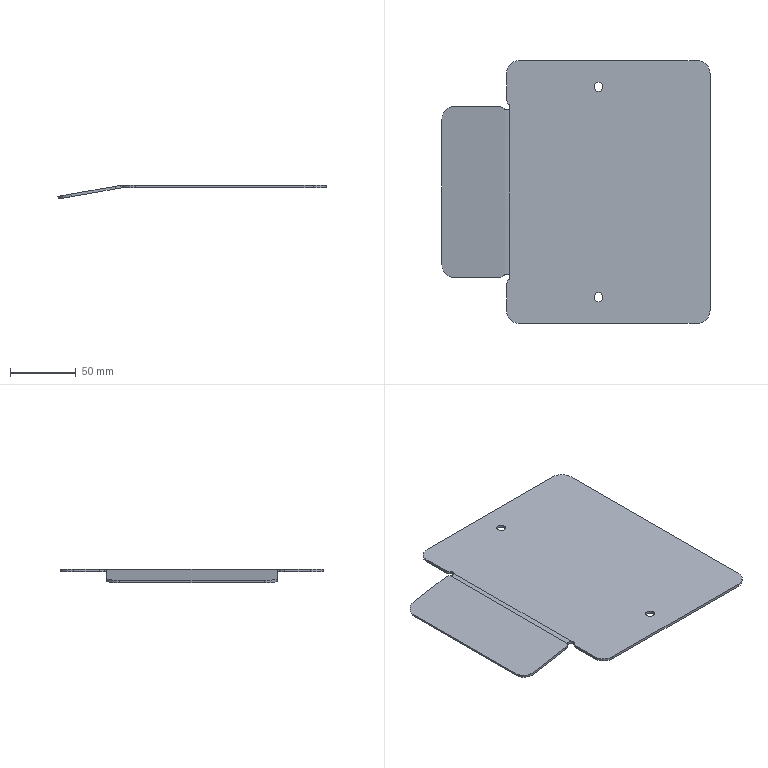Part | STEP file | 冲床-300配套压波_id882_x_t | 1 solid | 28 faces | box 204.24 x 200 x 10.652 mm | volume 74480 mm3 | plane 12 | cylinder 10 | spline 6 | commonest cylinder face diameters 20 x6 6.8 x2 40 x1 44 x1
STEP:
#1=CARTESIAN_POINT('',(1395.4,-80.,142.083));
#2=VERTEX_POINT('',#1);
#3=CARTESIAN_POINT('',(1392.,-80.,142.083));
#4=DIRECTION('',(0.,0.,-1.));
#5=DIRECTION('',(1.,0.,0.));
#6=AXIS2_PLACEMENT_3D('',#3,#4,#5);
#7=CIRCLE('',#6,3.4);
#8=EDGE_CURVE('',#2,#2,#7,.T.);
#9=ORIENTED_EDGE('',*,*,#8,.F.);
#10=EDGE_LOOP('',(#9));
#11=FACE_BOUND('',#10,.T.);
#12=CARTESIAN_POINT('',(1395.4,80.,142.083));
#13=VERTEX_POINT('',#12);
#14=CARTESIAN_POINT('',(1392.,80.,142.083));
#15=DIRECTION('',(0.,0.,1.));
#16=DIRECTION('',(1.,0.,0.));
#17=AXIS2_PLACEMENT_3D('',#14,#15,#16);
#18=CIRCLE('',#17,3.4);
#19=EDGE_CURVE('',#13,#13,#18,.T.);
#20=ORIENTED_EDGE('',*,*,#19,.T.);
#21=EDGE_LOOP('',(#20));
#22=FACE_BOUND('',#21,.T.);
#23=CARTESIAN_POINT('',(1323.925,-63.405,142.083));
#24=VERTEX_POINT('',#23);
#25=CARTESIAN_POINT('',(1323.667,-66.863,142.083));
#26=VERTEX_POINT('',#25);
#27=CARTESIAN_POINT('',(1322.,-65.,142.083));
#28=DIRECTION('',(0.,0.,-1.));
#29=DIRECTION('',(1.,0.,0.));
#30=AXIS2_PLACEMENT_3D('',#27,#28,#29);
#31=CIRCLE('',#30,2.5);
#32=EDGE_CURVE('',#24,#26,#31,.T.);
#33=ORIENTED_EDGE('',*,*,#32,.F.);
#34=CARTESIAN_POINT('',(1323.925,63.405,142.083));
#35=VERTEX_POINT('',#34);
#36=CARTESIAN_POINT('',(1323.925,62.506,142.083));
#37=DIRECTION('',(0.,1.,0.));
#38=VECTOR('',#37,1.);
#39=LINE('',#36,#38);
#40=EDGE_CURVE('',#24,#35,#39,.T.);
#41=ORIENTED_EDGE('',*,*,#40,.T.);
#42=CARTESIAN_POINT('',(1323.667,66.863,142.083));
#43=VERTEX_POINT('',#42);
#44=CARTESIAN_POINT('',(1322.,65.,142.083));
#45=DIRECTION('',(0.,0.,-1.));
#46=DIRECTION('',(1.,0.,0.));
#47=AXIS2_PLACEMENT_3D('',#44,#45,#46);
#48=CIRCLE('',#47,2.5);
#49=EDGE_CURVE('',#43,#35,#48,.T.);
#50=ORIENTED_EDGE('',*,*,#49,.F.);
#51=CARTESIAN_POINT('',(1322.,70.59,142.083));
#52=VERTEX_POINT('',#51);
#53=CARTESIAN_POINT('',(1327.,70.59,142.083));
#54=DIRECTION('',(0.,0.,-1.));
#55=DIRECTION('',(1.,0.,0.));
#56=AXIS2_PLACEMENT_3D('',#53,#54,#55);
#57=CIRCLE('',#56,5.);
#58=EDGE_CURVE('',#43,#52,#57,.T.);
#59=ORIENTED_EDGE('',*,*,#58,.T.);
#60=CARTESIAN_POINT('',(1322.,90.,142.083));
#61=VERTEX_POINT('',#60);
#62=CARTESIAN_POINT('',(1322.,90.,142.083));
#63=DIRECTION('',(0.,-1.,0.));
#64=VECTOR('',#63,1.);
#65=LINE('',#62,#64);
#66=EDGE_CURVE('',#61,#52,#65,.T.);
#67=ORIENTED_EDGE('',*,*,#66,.F.);
#68=CARTESIAN_POINT('',(1332.,100.,142.083));
#69=VERTEX_POINT('',#68);
#70=CARTESIAN_POINT('',(1332.,90.,142.083));
#71=DIRECTION('',(0.,0.,-1.));
#72=DIRECTION('',(1.,0.,0.));
#73=AXIS2_PLACEMENT_3D('',#70,#71,#72);
#74=CIRCLE('',#73,10.);
#75=EDGE_CURVE('',#61,#69,#74,.T.);
#76=ORIENTED_EDGE('',*,*,#75,.T.);
#77=CARTESIAN_POINT('',(1467.,100.,142.083));
#78=VERTEX_POINT('',#77);
#79=CARTESIAN_POINT('',(1457.,100.,142.083));
#80=DIRECTION('',(-1.,0.,0.));
#81=VECTOR('',#80,1.);
#82=LINE('',#79,#81);
#83=EDGE_CURVE('',#78,#69,#82,.T.);
#84=ORIENTED_EDGE('',*,*,#83,.F.);
#85=CARTESIAN_POINT('',(1477.,90.,142.083));
#86=VERTEX_POINT('',#85);
#87=CARTESIAN_POINT('',(1467.,90.,142.083));
#88=DIRECTION('',(0.,0.,-1.));
#89=DIRECTION('',(1.,0.,0.));
#90=AXIS2_PLACEMENT_3D('',#87,#88,#89);
#91=CIRCLE('',#90,10.);
#92=EDGE_CURVE('',#78,#86,#91,.T.);
#93=ORIENTED_EDGE('',*,*,#92,.T.);
#94=CARTESIAN_POINT('',(1477.,-90.,142.083));
#95=VERTEX_POINT('',#94);
#96=CARTESIAN_POINT('',(1477.,-90.,142.083));
#97=DIRECTION('',(0.,1.,0.));
#98=VECTOR('',#97,1.);
#99=LINE('',#96,#98);
#100=EDGE_CURVE('',#95,#86,#99,.T.);
#101=ORIENTED_EDGE('',*,*,#100,.F.);
#102=CARTESIAN_POINT('',(1467.,-100.,142.083));
#103=VERTEX_POINT('',#102);
#104=CARTESIAN_POINT('',(1467.,-90.,142.083));
#105=DIRECTION('',(0.,0.,-1.));
#106=DIRECTION('',(1.,0.,0.));
#107=AXIS2_PLACEMENT_3D('',#104,#105,#106);
#108=CIRCLE('',#107,10.);
#109=EDGE_CURVE('',#95,#103,#108,.T.);
#110=ORIENTED_EDGE('',*,*,#109,.T.);
#111=CARTESIAN_POINT('',(1332.,-100.,142.083));
#112=VERTEX_POINT('',#111);
#113=CARTESIAN_POINT('',(1327.,-100.,142.083));
#114=DIRECTION('',(1.,0.,0.));
#115=VECTOR('',#114,1.);
#116=LINE('',#113,#115);
#117=EDGE_CURVE('',#112,#103,#116,.T.);
#118=ORIENTED_EDGE('',*,*,#117,.F.);
#119=CARTESIAN_POINT('',(1322.,-90.,142.083));
#120=VERTEX_POINT('',#119);
#121=CARTESIAN_POINT('',(1332.,-90.,142.083));
#122=DIRECTION('',(0.,0.,-1.));
#123=DIRECTION('',(1.,0.,0.));
#124=AXIS2_PLACEMENT_3D('',#121,#122,#123);
#125=CIRCLE('',#124,10.);
#126=EDGE_CURVE('',#112,#120,#125,.T.);
#127=ORIENTED_EDGE('',*,*,#126,.T.);
#128=CARTESIAN_POINT('',(1322.,-70.59,142.083));
#129=VERTEX_POINT('',#128);
#130=CARTESIAN_POINT('',(1322.,90.,142.083));
#131=DIRECTION('',(0.,-1.,0.));
#132=VECTOR('',#131,1.);
#133=LINE('',#130,#132);
#134=EDGE_CURVE('',#129,#120,#133,.T.);
#135=ORIENTED_EDGE('',*,*,#134,.F.);
#136=CARTESIAN_POINT('',(1327.,-70.59,142.083));
#137=DIRECTION('',(0.,0.,-1.));
#138=DIRECTION('',(1.,0.,0.));
#139=AXIS2_PLACEMENT_3D('',#136,#137,#138);
#140=CIRCLE('',#139,5.);
#141=EDGE_CURVE('',#129,#26,#140,.T.);
#142=ORIENTED_EDGE('',*,*,#141,.T.);
#143=EDGE_LOOP('',(#33,#41,#50,#59,#67,#76,#84,#93,#101,#110,#118,#127,#135,#142));
#144=FACE_BOUND('',#143,.T.);
#145=CARTESIAN_POINT('',(-15.,0.,142.083));
#146=DIRECTION('',(0.,0.,1.));
#147=DIRECTION('',(1.,0.,0.));
#148=AXIS2_PLACEMENT_3D('',#145,#146,#147);
#149=PLANE('',#148);
#150=ADVANCED_FACE('',(#11,#22,#144),#149,.F.);
#151=CARTESIAN_POINT('',(1395.4,-80.,144.083));
#152=VERTEX_POINT('',#151);
#153=CARTESIAN_POINT('',(1392.,-80.,144.083));
#154=DIRECTION('',(0.,0.,-1.));
#155=DIRECTION('',(1.,0.,0.));
#156=AXIS2_PLACEMENT_3D('',#153,#154,#155);
#157=CIRCLE('',#156,3.4);
#158=EDGE_CURVE('',#152,#152,#157,.T.);
#159=ORIENTED_EDGE('',*,*,#158,.T.);
#160=EDGE_LOOP('',(#159));
#161=FACE_BOUND('',#160,.T.);
#162=CARTESIAN_POINT('',(1395.4,80.,144.083));
#163=VERTEX_POINT('',#162);
#164=CARTESIAN_POINT('',(1392.,80.,144.083));
#165=DIRECTION('',(0.,0.,1.));
#166=DIRECTION('',(1.,0.,0.));
#167=AXIS2_PLACEMENT_3D('',#164,#165,#166);
#168=CIRCLE('',#167,3.4);
#169=EDGE_CURVE('',#163,#163,#168,.T.);
#170=ORIENTED_EDGE('',*,*,#169,.F.);
#171=EDGE_LOOP('',(#170));
#172=FACE_BOUND('',#171,.T.);
#173=CARTESIAN_POINT('',(1323.925,63.405,144.083));
#174=VERTEX_POINT('',#173);
#175=CARTESIAN_POINT('',(1323.667,66.863,144.083));
#176=VERTEX_POINT('',#175);
#177=CARTESIAN_POINT('',(1323.925,63.405,144.083));
#178=CARTESIAN_POINT('',(1324.217,63.757,144.083));
#179=CARTESIAN_POINT('',(1324.417,64.172,144.083));
#180=CARTESIAN_POINT('',(1324.5,64.608,144.083));
#181=CARTESIAN_POINT('',(1324.5,65.,144.083));
#182=CARTESIAN_POINT('',(1324.5,65.472,144.083));
#183=CARTESIAN_POINT('',(1324.379,66.009,144.083));
#184=CARTESIAN_POINT('',(1324.079,66.495,144.083));
#185=CARTESIAN_POINT('',(1323.667,66.863,144.083));
#186=(BOUNDED_CURVE()B_SPLINE_CURVE(4,(#177,#178,#179,#180,#181,#182,#183,#184,#185),.UNSPECIFIED.,.F.,.F.)B_SPLINE_CURVE_WITH_KNOTS((5,4,5),(0.,0.454,1.),.UNSPECIFIED.)CURVE()GEOMETRIC_REPRESENTATION_ITEM()RATIONAL_B_SPLINE_CURVE((0.9954,0.9975,1.005,1.017,1.017,1.017,1.,0.9934,0.995))REPRESENTATION_ITEM(''));
#187=EDGE_CURVE('',#174,#176,#186,.T.);
#188=ORIENTED_EDGE('',*,*,#187,.F.);
#189=CARTESIAN_POINT('',(1323.925,-63.405,144.083));
#190=VERTEX_POINT('',#189);
#191=CARTESIAN_POINT('',(1323.925,0.,144.083));
#192=DIRECTION('',(0.,-1.,0.));
#193=VECTOR('',#192,1.);
#194=LINE('',#191,#193);
#195=EDGE_CURVE('',#174,#190,#194,.T.);
#196=ORIENTED_EDGE('',*,*,#195,.T.);
#197=CARTESIAN_POINT('',(1323.667,-66.863,144.083));
#198=VERTEX_POINT('',#197);
#199=CARTESIAN_POINT('',(1323.667,-66.863,144.083));
#200=CARTESIAN_POINT('',(1324.079,-66.495,144.083));
#201=CARTESIAN_POINT('',(1324.379,-66.009,144.083));
#202=CARTESIAN_POINT('',(1324.5,-65.472,144.083));
#203=CARTESIAN_POINT('',(1324.5,-65.,144.083));
#204=CARTESIAN_POINT('',(1324.5,-64.608,144.083));
#205=CARTESIAN_POINT('',(1324.417,-64.172,144.083));
#206=CARTESIAN_POINT('',(1324.217,-63.757,144.083));
#207=CARTESIAN_POINT('',(1323.925,-63.405,144.083));
#208=(BOUNDED_CURVE()B_SPLINE_CURVE(4,(#199,#200,#201,#202,#203,#204,#205,#206,#207),.UNSPECIFIED.,.F.,.F.)B_SPLINE_CURVE_WITH_KNOTS((5,4,5),(0.,0.546,1.),.UNSPECIFIED.)CURVE()GEOMETRIC_REPRESENTATION_ITEM()RATIONAL_B_SPLINE_CURVE((0.995,0.9934,1.,1.017,1.017,1.017,1.005,0.9975,0.9954))REPRESENTATION_ITEM(''));
#209=EDGE_CURVE('',#198,#190,#208,.T.);
#210=ORIENTED_EDGE('',*,*,#209,.F.);
#211=CARTESIAN_POINT('',(1322.,-70.59,144.083));
#212=VERTEX_POINT('',#211);
#213=CARTESIAN_POINT('',(1327.,-70.59,144.083));
#214=DIRECTION('',(0.,0.,1.));
#215=DIRECTION('',(1.,0.,0.));
#216=AXIS2_PLACEMENT_3D('',#213,#214,#215);
#217=CIRCLE('',#216,5.);
#218=EDGE_CURVE('',#198,#212,#217,.T.);
#219=ORIENTED_EDGE('',*,*,#218,.T.);
#220=CARTESIAN_POINT('',(1322.,-90.,144.083));
#221=VERTEX_POINT('',#220);
#222=CARTESIAN_POINT('',(1322.,90.,144.083));
#223=DIRECTION('',(0.,-1.,0.));
#224=VECTOR('',#223,1.);
#225=LINE('',#222,#224);
#226=EDGE_CURVE('',#212,#221,#225,.T.);
#227=ORIENTED_EDGE('',*,*,#226,.T.);
#228=CARTESIAN_POINT('',(1332.,-100.,144.083));
#229=VERTEX_POINT('',#228);
#230=CARTESIAN_POINT('',(1332.,-90.,144.083));
#231=DIRECTION('',(0.,0.,1.));
#232=DIRECTION('',(1.,0.,0.));
#233=AXIS2_PLACEMENT_3D('',#230,#231,#232);
#234=CIRCLE('',#233,10.);
#235=EDGE_CURVE('',#221,#229,#234,.T.);
#236=ORIENTED_EDGE('',*,*,#235,.T.);
#237=CARTESIAN_POINT('',(1467.,-100.,144.083));
#238=VERTEX_POINT('',#237);
#239=CARTESIAN_POINT('',(1327.,-100.,144.083));
#240=DIRECTION('',(1.,0.,0.));
#241=VECTOR('',#240,1.);
#242=LINE('',#239,#241);
#243=EDGE_CURVE('',#229,#238,#242,.T.);
#244=ORIENTED_EDGE('',*,*,#243,.T.);
#245=CARTESIAN_POINT('',(1477.,-90.,144.083));
#246=VERTEX_POINT('',#245);
#247=CARTESIAN_POINT('',(1467.,-90.,144.083));
#248=DIRECTION('',(0.,0.,1.));
#249=DIRECTION('',(1.,0.,0.));
#250=AXIS2_PLACEMENT_3D('',#247,#248,#249);
#251=CIRCLE('',#250,10.);
#252=EDGE_CURVE('',#238,#246,#251,.T.);
#253=ORIENTED_EDGE('',*,*,#252,.T.);
#254=CARTESIAN_POINT('',(1477.,90.,144.083));
#255=VERTEX_POINT('',#254);
#256=CARTESIAN_POINT('',(1477.,-90.,144.083));
#257=DIRECTION('',(0.,1.,0.));
#258=VECTOR('',#257,1.);
#259=LINE('',#256,#258);
#260=EDGE_CURVE('',#246,#255,#259,.T.);
#261=ORIENTED_EDGE('',*,*,#260,.T.);
#262=CARTESIAN_POINT('',(1467.,100.,144.083));
#263=VERTEX_POINT('',#262);
#264=CARTESIAN_POINT('',(1467.,90.,144.083));
#265=DIRECTION('',(0.,0.,1.));
#266=DIRECTION('',(1.,0.,0.));
#267=AXIS2_PLACEMENT_3D('',#264,#265,#266);
#268=CIRCLE('',#267,10.);
#269=EDGE_CURVE('',#255,#263,#268,.T.);
#270=ORIENTED_EDGE('',*,*,#269,.T.);
#271=CARTESIAN_POINT('',(1332.,100.,144.083));
#272=VERTEX_POINT('',#271);
#273=CARTESIAN_POINT('',(1457.,100.,144.083));
#274=DIRECTION('',(-1.,0.,0.));
#275=VECTOR('',#274,1.);
#276=LINE('',#273,#275);
#277=EDGE_CURVE('',#263,#272,#276,.T.);
#278=ORIENTED_EDGE('',*,*,#277,.T.);
#279=CARTESIAN_POINT('',(1322.,90.,144.083));
#280=VERTEX_POINT('',#279);
#281=CARTESIAN_POINT('',(1332.,90.,144.083));
#282=DIRECTION('',(0.,0.,1.));
#283=DIRECTION('',(1.,0.,0.));
#284=AXIS2_PLACEMENT_3D('',#281,#282,#283);
#285=CIRCLE('',#284,10.);
#286=EDGE_CURVE('',#272,#280,#285,.T.);
#287=ORIENTED_EDGE('',*,*,#286,.T.);
#288=CARTESIAN_POINT('',(1322.,70.59,144.083));
#289=VERTEX_POINT('',#288);
#290=CARTESIAN_POINT('',(1322.,90.,144.083));
#291=DIRECTION('',(0.,-1.,0.));
#292=VECTOR('',#291,1.);
#293=LINE('',#290,#292);
#294=EDGE_CURVE('',#280,#289,#293,.T.);
#295=ORIENTED_EDGE('',*,*,#294,.T.);
#296=CARTESIAN_POINT('',(1327.,70.59,144.083));
#297=DIRECTION('',(0.,0.,1.));
#298=DIRECTION('',(1.,0.,0.));
#299=AXIS2_PLACEMENT_3D('',#296,#297,#298);
#300=CIRCLE('',#299,5.);
#301=EDGE_CURVE('',#289,#176,#300,.T.);
#302=ORIENTED_EDGE('',*,*,#301,.T.);
#303=EDGE_LOOP('',(#188,#196,#210,#219,#227,#236,#244,#253,#261,#270,#278,#287,#295,#302));
#304=FACE_BOUND('',#303,.T.);
#305=CARTESIAN_POINT('',(-15.,0.,144.083));
#306=DIRECTION('',(0.,0.,1.));
#307=DIRECTION('',(1.,0.,0.));
#308=AXIS2_PLACEMENT_3D('',#305,#306,#307);
#309=PLANE('',#308);
#310=ADVANCED_FACE('',(#161,#172,#304),#309,.T.);
#311=CARTESIAN_POINT('',(1316.41,-65.,143.098));
#312=VERTEX_POINT('',#311);
#313=CARTESIAN_POINT('',(1320.104,-63.369,143.749));
#314=VERTEX_POINT('',#313);
#315=CARTESIAN_POINT('',(1316.41,-65.,143.098));
#316=CARTESIAN_POINT('',(1317.803,-65.,143.343));
#317=CARTESIAN_POINT('',(1319.159,-64.406,143.582));
#318=CARTESIAN_POINT('',(1320.104,-63.369,143.749));
#319=B_SPLINE_CURVE_WITH_KNOTS('',3,(#315,#316,#317,#318),.UNSPECIFIED.,.F.,.F.,(4,4),(0.,1.),.UNSPECIFIED.);
#320=EDGE_CURVE('',#312,#314,#319,.T.);
#321=ORIENTED_EDGE('',*,*,#320,.T.);
#322=CARTESIAN_POINT('',(1320.104,63.369,143.749));
#323=VERTEX_POINT('',#322);
#324=CARTESIAN_POINT('',(1320.104,0.,143.749));
#325=DIRECTION('',(0.,1.,0.));
#326=VECTOR('',#325,1.);
#327=LINE('',#324,#326);
#328=EDGE_CURVE('',#314,#323,#327,.T.);
#329=ORIENTED_EDGE('',*,*,#328,.T.);
#330=CARTESIAN_POINT('',(1316.41,65.,143.098));
#331=VERTEX_POINT('',#330);
#332=CARTESIAN_POINT('',(1320.104,63.369,143.749));
#333=CARTESIAN_POINT('',(1319.16,64.405,143.583));
#334=CARTESIAN_POINT('',(1317.803,65.,143.343));
#335=CARTESIAN_POINT('',(1316.41,65.,143.098));
#336=B_SPLINE_CURVE_WITH_KNOTS('',3,(#332,#333,#334,#335),.UNSPECIFIED.,.F.,.F.,(4,4),(0.,1.),.UNSPECIFIED.);
#337=EDGE_CURVE('',#323,#331,#336,.T.);
#338=ORIENTED_EDGE('',*,*,#337,.T.);
#339=CARTESIAN_POINT('',(1282.608,65.,137.138));
#340=VERTEX_POINT('',#339);
#341=CARTESIAN_POINT('',(5.312,65.,-88.084));
#342=DIRECTION('',(-0.9848,0.,-0.1736));
#343=VECTOR('',#342,1.);
#344=LINE('',#341,#343);
#345=EDGE_CURVE('',#331,#340,#344,.T.);
#346=ORIENTED_EDGE('',*,*,#345,.T.);
#347=CARTESIAN_POINT('',(1272.76,55.,135.401));
#348=VERTEX_POINT('',#347);
#349=CARTESIAN_POINT('',(1282.608,55.,137.138));
#350=DIRECTION('',(-0.1736,0.,0.9848));
#351=DIRECTION('',(0.9848,0.,0.1736));
#352=AXIS2_PLACEMENT_3D('',#349,#350,#351);
#353=CIRCLE('',#352,10.);
#354=EDGE_CURVE('',#340,#348,#353,.T.);
#355=ORIENTED_EDGE('',*,*,#354,.T.);
#356=CARTESIAN_POINT('',(1272.76,-55.,135.401));
#357=VERTEX_POINT('',#356);
#358=CARTESIAN_POINT('',(1272.76,0.,135.401));
#359=DIRECTION('',(0.,1.,0.));
#360=VECTOR('',#359,1.);
#361=LINE('',#358,#360);
#362=EDGE_CURVE('',#357,#348,#361,.T.);
#363=ORIENTED_EDGE('',*,*,#362,.F.);
#364=CARTESIAN_POINT('',(1282.608,-65.,137.138));
#365=VERTEX_POINT('',#364);
#366=CARTESIAN_POINT('',(1282.608,-55.,137.138));
#367=DIRECTION('',(-0.1736,0.,0.9848));
#368=DIRECTION('',(0.9848,0.,0.1736));
#369=AXIS2_PLACEMENT_3D('',#366,#367,#368);
#370=CIRCLE('',#369,10.);
#371=EDGE_CURVE('',#357,#365,#370,.T.);
#372=ORIENTED_EDGE('',*,*,#371,.T.);
#373=CARTESIAN_POINT('',(5.312,-65.,-88.084));
#374=DIRECTION('',(0.9848,0.,0.1736));
#375=VECTOR('',#374,1.);
#376=LINE('',#373,#375);
#377=EDGE_CURVE('',#365,#312,#376,.T.);
#378=ORIENTED_EDGE('',*,*,#377,.T.);
#379=EDGE_LOOP('',(#321,#329,#338,#346,#355,#363,#372,#378));
#380=FACE_OUTER_BOUND('',#379,.T.);
#381=CARTESIAN_POINT('',(5.312,0.,-88.084));
#382=DIRECTION('',(-0.1736,0.,0.9848));
#383=DIRECTION('',(0.9848,0.,0.1736));
#384=AXIS2_PLACEMENT_3D('',#381,#382,#383);
#385=PLANE('',#384);
#386=ADVANCED_FACE('',(#380),#385,.T.);
#387=ORIENTED_EDGE('',*,*,#66,.T.);
#388=CARTESIAN_POINT('',(1322.,70.59,142.083));
#389=CARTESIAN_POINT('',(1322.,70.59,142.1));
#390=CARTESIAN_POINT('',(1322.,70.59,142.117));
#391=CARTESIAN_POINT('',(1322.,70.59,142.134));
#392=CARTESIAN_POINT('',(1322.,70.59,142.368));
#393=CARTESIAN_POINT('',(1322.,70.59,142.602));
#394=CARTESIAN_POINT('',(1322.,70.59,142.836));
#395=CARTESIAN_POINT('',(1322.,70.59,143.148));
#396=CARTESIAN_POINT('',(1322.,70.59,143.46));
#397=CARTESIAN_POINT('',(1322.,70.59,143.772));
#398=CARTESIAN_POINT('',(1322.,70.59,143.876));
#399=CARTESIAN_POINT('',(1322.,70.59,143.98));
#400=CARTESIAN_POINT('',(1322.,70.59,144.083));
#401=B_SPLINE_CURVE_WITH_KNOTS('',3,(#388,#389,#390,#391,#392,#393,#394,#395,#396,#397,#398,#399,#400),.UNSPECIFIED.,.F.,.F.,(4,3,3,3,4),(0.,0.02529,0.3762,0.844,1.),.UNSPECIFIED.);
#402=EDGE_CURVE('',#52,#289,#401,.T.);
#403=ORIENTED_EDGE('',*,*,#402,.T.);
#404=ORIENTED_EDGE('',*,*,#294,.F.);
#405=CARTESIAN_POINT('',(1322.,90.,126.083));
#406=DIRECTION('',(0.,0.,-1.));
#407=VECTOR('',#406,1.);
#408=LINE('',#405,#407);
#409=EDGE_CURVE('',#280,#61,#408,.T.);
#410=ORIENTED_EDGE('',*,*,#409,.T.);
#411=EDGE_LOOP('',(#387,#403,#404,#410));
#412=FACE_OUTER_BOUND('',#411,.T.);
#413=CARTESIAN_POINT('',(1322.,90.,126.083));
#414=DIRECTION('',(1.,0.,0.));
#415=DIRECTION('',(0.,0.,-1.));
#416=AXIS2_PLACEMENT_3D('',#413,#414,#415);
#417=PLANE('',#416);
#418=ADVANCED_FACE('',(#412),#417,.F.);
#419=ORIENTED_EDGE('',*,*,#345,.F.);
#420=CARTESIAN_POINT('',(1316.41,65.,141.067));
#421=VERTEX_POINT('',#420);
#422=CARTESIAN_POINT('',(1316.41,65.,143.098));
#423=CARTESIAN_POINT('',(1316.41,65.,142.864));
#424=CARTESIAN_POINT('',(1316.41,65.,142.629));
#425=CARTESIAN_POINT('',(1316.41,65.,142.395));
#426=CARTESIAN_POINT('',(1316.41,65.,142.17));
#427=CARTESIAN_POINT('',(1316.41,65.,141.946));
#428=CARTESIAN_POINT('',(1316.41,65.,141.721));
#429=CARTESIAN_POINT('',(1316.41,65.,141.503));
#430=CARTESIAN_POINT('',(1316.41,65.,141.285));
#431=CARTESIAN_POINT('',(1316.41,65.,141.067));
#432=B_SPLINE_CURVE_WITH_KNOTS('',3,(#422,#423,#424,#425,#426,#427,#428,#429,#430,#431),.UNSPECIFIED.,.F.,.F.,(4,3,3,4),(0.,0.346,0.678,1.),.UNSPECIFIED.);
#433=EDGE_CURVE('',#331,#421,#432,.T.);
#434=ORIENTED_EDGE('',*,*,#433,.T.);
#435=CARTESIAN_POINT('',(1282.955,65.,135.168));
#436=VERTEX_POINT('',#435);
#437=CARTESIAN_POINT('',(1322.347,65.,142.114));
#438=DIRECTION('',(0.9848,0.,0.1736));
#439=VECTOR('',#438,1.);
#440=LINE('',#437,#439);
#441=EDGE_CURVE('',#436,#421,#440,.T.);
#442=ORIENTED_EDGE('',*,*,#441,.F.);
#443=CARTESIAN_POINT('',(1303.512,65.,18.583));
#444=DIRECTION('',(-0.1736,0.,0.9848));
#445=VECTOR('',#444,1.);
#446=LINE('',#443,#445);
#447=EDGE_CURVE('',#436,#340,#446,.T.);
#448=ORIENTED_EDGE('',*,*,#447,.T.);
#449=EDGE_LOOP('',(#419,#434,#442,#448));
#450=FACE_OUTER_BOUND('',#449,.T.);
#451=CARTESIAN_POINT('',(1331.087,65.,23.445));
#452=DIRECTION('',(0.,1.,0.));
#453=DIRECTION('',(-0.9848,0.,-0.1736));
#454=AXIS2_PLACEMENT_3D('',#451,#452,#453);
#455=PLANE('',#454);
#456=ADVANCED_FACE('',(#450),#455,.T.);
#457=ORIENTED_EDGE('',*,*,#226,.F.);
#458=CARTESIAN_POINT('',(1322.,-70.59,144.083));
#459=CARTESIAN_POINT('',(1322.,-70.59,144.056));
#460=CARTESIAN_POINT('',(1322.,-70.59,144.029));
#461=CARTESIAN_POINT('',(1322.,-70.59,144.002));
#462=CARTESIAN_POINT('',(1322.,-70.59,143.778));
#463=CARTESIAN_POINT('',(1322.,-70.59,143.555));
#464=CARTESIAN_POINT('',(1322.,-70.59,143.331));
#465=CARTESIAN_POINT('',(1322.,-70.59,143.019));
#466=CARTESIAN_POINT('',(1322.,-70.59,142.707));
#467=CARTESIAN_POINT('',(1322.,-70.59,142.395));
#468=CARTESIAN_POINT('',(1322.,-70.59,142.291));
#469=CARTESIAN_POINT('',(1322.,-70.59,142.187));
#470=CARTESIAN_POINT('',(1322.,-70.59,142.083));
#471=B_SPLINE_CURVE_WITH_KNOTS('',3,(#458,#459,#460,#461,#462,#463,#464,#465,#466,#467,#468,#469,#470),.UNSPECIFIED.,.F.,.F.,(4,3,3,3,4),(0.,0.04077,0.3762,0.844,1.),.UNSPECIFIED.);
#472=EDGE_CURVE('',#212,#129,#471,.T.);
#473=ORIENTED_EDGE('',*,*,#472,.T.);
#474=ORIENTED_EDGE('',*,*,#134,.T.);
#475=CARTESIAN_POINT('',(1322.,-90.,126.083));
#476=DIRECTION('',(0.,0.,1.));
#477=VECTOR('',#476,1.);
#478=LINE('',#475,#477);
#479=EDGE_CURVE('',#120,#221,#478,.T.);
#480=ORIENTED_EDGE('',*,*,#479,.T.);
#481=EDGE_LOOP('',(#457,#473,#474,#480));
#482=FACE_OUTER_BOUND('',#481,.T.);
#483=CARTESIAN_POINT('',(1322.,90.,126.083));
#484=DIRECTION('',(1.,0.,0.));
#485=DIRECTION('',(0.,0.,-1.));
#486=AXIS2_PLACEMENT_3D('',#483,#484,#485);
#487=PLANE('',#486);
#488=ADVANCED_FACE('',(#482),#487,.F.);
#489=CARTESIAN_POINT('',(1316.41,-65.,141.067));
#490=VERTEX_POINT('',#489);
#491=CARTESIAN_POINT('',(1282.955,-65.,135.168));
#492=VERTEX_POINT('',#491);
#493=CARTESIAN_POINT('',(1322.347,-65.,142.114));
#494=DIRECTION('',(-0.9848,0.,-0.1736));
#495=VECTOR('',#494,1.);
#496=LINE('',#493,#495);
#497=EDGE_CURVE('',#490,#492,#496,.T.);
#498=ORIENTED_EDGE('',*,*,#497,.F.);
#499=CARTESIAN_POINT('',(1316.41,-65.,141.067));
#500=CARTESIAN_POINT('',(1316.41,-65.,141.151));
#501=CARTESIAN_POINT('',(1316.41,-65.,141.235));
#502=CARTESIAN_POINT('',(1316.41,-65.,141.32));
#503=CARTESIAN_POINT('',(1316.41,-65.,141.551));
#504=CARTESIAN_POINT('',(1316.41,-65.,141.782));
#505=CARTESIAN_POINT('',(1316.41,-65.,142.014));
#506=CARTESIAN_POINT('',(1316.41,-65.,142.245));
#507=CARTESIAN_POINT('',(1316.41,-65.,142.476));
#508=CARTESIAN_POINT('',(1316.41,-65.,142.707));
#509=CARTESIAN_POINT('',(1316.41,-65.,142.837));
#510=CARTESIAN_POINT('',(1316.41,-65.,142.968));
#511=CARTESIAN_POINT('',(1316.41,-65.,143.098));
#512=B_SPLINE_CURVE_WITH_KNOTS('',3,(#499,#500,#501,#502,#503,#504,#505,#506,#507,#508,#509,#510,#511),.UNSPECIFIED.,.F.,.F.,(4,3,3,3,4),(0.,0.1245,0.4661,0.8077,1.),.UNSPECIFIED.);
#513=EDGE_CURVE('',#490,#312,#512,.T.);
#514=ORIENTED_EDGE('',*,*,#513,.T.);
#515=ORIENTED_EDGE('',*,*,#377,.F.);
#516=CARTESIAN_POINT('',(1303.512,-65.,18.583));
#517=DIRECTION('',(0.1736,0.,-0.9848));
#518=VECTOR('',#517,1.);
#519=LINE('',#516,#518);
#520=EDGE_CURVE('',#365,#492,#519,.T.);
#521=ORIENTED_EDGE('',*,*,#520,.T.);
#522=EDGE_LOOP('',(#498,#514,#515,#521));
#523=FACE_OUTER_BOUND('',#522,.T.);
#524=CARTESIAN_POINT('',(1331.087,-65.,23.445));
#525=DIRECTION('',(0.,-1.,0.));
#526=DIRECTION('',(-0.9848,0.,-0.1736));
#527=AXIS2_PLACEMENT_3D('',#524,#525,#526);
#528=PLANE('',#527);
#529=ADVANCED_FACE('',(#523),#528,.T.);
#530=ORIENTED_EDGE('',*,*,#243,.F.);
#531=CARTESIAN_POINT('',(1332.,-100.,126.083));
#532=DIRECTION('',(0.,0.,-1.));
#533=VECTOR('',#532,1.);
#534=LINE('',#531,#533);
#535=EDGE_CURVE('',#229,#112,#534,.T.);
#536=ORIENTED_EDGE('',*,*,#535,.T.);
#537=ORIENTED_EDGE('',*,*,#117,.T.);
#538=CARTESIAN_POINT('',(1467.,-100.,126.083));
#539=DIRECTION('',(0.,0.,1.));
#540=VECTOR('',#539,1.);
#541=LINE('',#538,#540);
#542=EDGE_CURVE('',#103,#238,#541,.T.);
#543=ORIENTED_EDGE('',*,*,#542,.T.);
#544=EDGE_LOOP('',(#530,#536,#537,#543));
#545=FACE_OUTER_BOUND('',#544,.T.);
#546=CARTESIAN_POINT('',(1327.,-100.,126.083));
#547=DIRECTION('',(0.,1.,0.));
#548=DIRECTION('',(0.,0.,1.));
#549=AXIS2_PLACEMENT_3D('',#546,#547,#548);
#550=PLANE('',#549);
#551=ADVANCED_FACE('',(#545),#550,.F.);
#552=ORIENTED_EDGE('',*,*,#260,.F.);
#553=CARTESIAN_POINT('',(1477.,-90.,126.083));
#554=DIRECTION('',(0.,0.,-1.));
#555=VECTOR('',#554,1.);
#556=LINE('',#553,#555);
#557=EDGE_CURVE('',#246,#95,#556,.T.);
#558=ORIENTED_EDGE('',*,*,#557,.T.);
#559=ORIENTED_EDGE('',*,*,#100,.T.);
#560=CARTESIAN_POINT('',(1477.,90.,126.083));
#561=DIRECTION('',(0.,0.,1.));
#562=VECTOR('',#561,1.);
#563=LINE('',#560,#562);
#564=EDGE_CURVE('',#86,#255,#563,.T.);
#565=ORIENTED_EDGE('',*,*,#564,.T.);
#566=EDGE_LOOP('',(#552,#558,#559,#565));
#567=FACE_OUTER_BOUND('',#566,.T.);
#568=CARTESIAN_POINT('',(1477.,-90.,126.083));
#569=DIRECTION('',(-1.,0.,0.));
#570=DIRECTION('',(0.,0.,1.));
#571=AXIS2_PLACEMENT_3D('',#568,#569,#570);
#572=PLANE('',#571);
#573=ADVANCED_FACE('',(#567),#572,.F.);
#574=ORIENTED_EDGE('',*,*,#277,.F.);
#575=CARTESIAN_POINT('',(1467.,100.,126.083));
#576=DIRECTION('',(0.,0.,-1.));
#577=VECTOR('',#576,1.);
#578=LINE('',#575,#577);
#579=EDGE_CURVE('',#263,#78,#578,.T.);
#580=ORIENTED_EDGE('',*,*,#579,.T.);
#581=ORIENTED_EDGE('',*,*,#83,.T.);
#582=CARTESIAN_POINT('',(1332.,100.,126.083));
#583=DIRECTION('',(0.,0.,1.));
#584=VECTOR('',#583,1.);
#585=LINE('',#582,#584);
#586=EDGE_CURVE('',#69,#272,#585,.T.);
#587=ORIENTED_EDGE('',*,*,#586,.T.);
#588=EDGE_LOOP('',(#574,#580,#581,#587));
#589=FACE_OUTER_BOUND('',#588,.T.);
#590=CARTESIAN_POINT('',(1457.,100.,126.083));
#591=DIRECTION('',(0.,-1.,0.));
#592=DIRECTION('',(0.,0.,-1.));
#593=AXIS2_PLACEMENT_3D('',#590,#591,#592);
#594=PLANE('',#593);
#595=ADVANCED_FACE('',(#589),#594,.F.);
#596=ORIENTED_EDGE('',*,*,#158,.F.);
#597=EDGE_LOOP('',(#596));
#598=FACE_BOUND('',#597,.T.);
#599=ORIENTED_EDGE('',*,*,#8,.T.);
#600=EDGE_LOOP('',(#599));
#601=FACE_BOUND('',#600,.T.);
#602=CARTESIAN_POINT('',(1392.,-80.,-55.917));
#603=DIRECTION('',(0.,0.,1.));
#604=DIRECTION('',(1.,0.,0.));
#605=AXIS2_PLACEMENT_3D('',#602,#603,#604);
#606=CYLINDRICAL_SURFACE('',#605,3.4);
#607=ADVANCED_FACE('',(#598,#601),#606,.F.);
#608=ORIENTED_EDGE('',*,*,#169,.T.);
#609=EDGE_LOOP('',(#608));
#610=FACE_BOUND('',#609,.T.);
#611=ORIENTED_EDGE('',*,*,#19,.F.);
#612=EDGE_LOOP('',(#611));
#613=FACE_BOUND('',#612,.T.);
#614=CARTESIAN_POINT('',(1392.,80.,-55.917));
#615=DIRECTION('',(0.,0.,1.));
#616=DIRECTION('',(1.,0.,0.));
#617=AXIS2_PLACEMENT_3D('',#614,#615,#616);
#618=CYLINDRICAL_SURFACE('',#617,3.4);
#619=ADVANCED_FACE('',(#610,#613),#618,.F.);
#620=ORIENTED_EDGE('',*,*,#235,.F.);
#621=ORIENTED_EDGE('',*,*,#479,.F.);
#622=ORIENTED_EDGE('',*,*,#126,.F.);
#623=ORIENTED_EDGE('',*,*,#535,.F.);
#624=EDGE_LOOP('',(#620,#621,#622,#623));
#625=FACE_OUTER_BOUND('',#624,.T.);
#626=CARTESIAN_POINT('',(1332.,-90.,126.083));
#627=DIRECTION('',(0.,0.,-1.));
#628=DIRECTION('',(-1.,0.,0.));
#629=AXIS2_PLACEMENT_3D('',#626,#627,#628);
#630=CYLINDRICAL_SURFACE('',#629,10.);
#631=ADVANCED_FACE('',(#625),#630,.T.);
#632=ORIENTED_EDGE('',*,*,#252,.F.);
#633=ORIENTED_EDGE('',*,*,#542,.F.);
#634=ORIENTED_EDGE('',*,*,#109,.F.);
#635=ORIENTED_EDGE('',*,*,#557,.F.);
#636=EDGE_LOOP('',(#632,#633,#634,#635));
#637=FACE_OUTER_BOUND('',#636,.T.);
#638=CARTESIAN_POINT('',(1467.,-90.,126.083));
#639=DIRECTION('',(0.,0.,-1.));
#640=DIRECTION('',(-1.,0.,0.));
#641=AXIS2_PLACEMENT_3D('',#638,#639,#640);
#642=CYLINDRICAL_SURFACE('',#641,10.);
#643=ADVANCED_FACE('',(#637),#642,.T.);
#644=ORIENTED_EDGE('',*,*,#269,.F.);
#645=ORIENTED_EDGE('',*,*,#564,.F.);
#646=ORIENTED_EDGE('',*,*,#92,.F.);
#647=ORIENTED_EDGE('',*,*,#579,.F.);
#648=EDGE_LOOP('',(#644,#645,#646,#647));
#649=FACE_OUTER_BOUND('',#648,.T.);
#650=CARTESIAN_POINT('',(1467.,90.,126.083));
#651=DIRECTION('',(0.,0.,-1.));
#652=DIRECTION('',(-1.,0.,0.));
#653=AXIS2_PLACEMENT_3D('',#650,#651,#652);
#654=CYLINDRICAL_SURFACE('',#653,10.);
#655=ADVANCED_FACE('',(#649),#654,.T.);
#656=ORIENTED_EDGE('',*,*,#286,.F.);
#657=ORIENTED_EDGE('',*,*,#586,.F.);
#658=ORIENTED_EDGE('',*,*,#75,.F.);
#659=ORIENTED_EDGE('',*,*,#409,.F.);
#660=EDGE_LOOP('',(#656,#657,#658,#659));
#661=FACE_OUTER_BOUND('',#660,.T.);
#662=CARTESIAN_POINT('',(1332.,90.,126.083));
#663=DIRECTION('',(0.,0.,-1.));
#664=DIRECTION('',(-1.,0.,0.));
#665=AXIS2_PLACEMENT_3D('',#662,#663,#664);
#666=CYLINDRICAL_SURFACE('',#665,10.);
#667=ADVANCED_FACE('',(#661),#666,.T.);
#668=CARTESIAN_POINT('',(1320.137,63.333,141.724));
#669=VERTEX_POINT('',#668);
#670=CARTESIAN_POINT('',(1320.452,63.037,141.78));
#671=VERTEX_POINT('',#670);
#672=CARTESIAN_POINT('',(1320.137,63.333,141.724));
#673=CARTESIAN_POINT('',(1320.233,63.226,141.741));
#674=CARTESIAN_POINT('',(1320.339,63.126,141.76));
#675=CARTESIAN_POINT('',(1320.452,63.037,141.78));
#676=B_SPLINE_CURVE_WITH_KNOTS('',3,(#672,#673,#674,#675),.UNSPECIFIED.,.F.,.F.,(4,4),(0.,1.),.UNSPECIFIED.);
#677=EDGE_CURVE('',#669,#671,#676,.T.);
#678=ORIENTED_EDGE('',*,*,#677,.T.);
#679=CARTESIAN_POINT('',(1320.452,-63.037,141.78));
#680=VERTEX_POINT('',#679);
#681=CARTESIAN_POINT('',(1320.452,-62.506,141.78));
#682=DIRECTION('',(0.,-1.,0.));
#683=VECTOR('',#682,1.);
#684=LINE('',#681,#683);
#685=EDGE_CURVE('',#671,#680,#684,.T.);
#686=ORIENTED_EDGE('',*,*,#685,.T.);
#687=CARTESIAN_POINT('',(1320.137,-63.333,141.724));
#688=VERTEX_POINT('',#687);
#689=CARTESIAN_POINT('',(1320.452,-63.037,141.78));
#690=CARTESIAN_POINT('',(1320.442,-63.045,141.778));
#691=CARTESIAN_POINT('',(1320.432,-63.053,141.776));
#692=CARTESIAN_POINT('',(1320.422,-63.061,141.774));
#693=CARTESIAN_POINT('',(1320.32,-63.144,141.756));
#694=CARTESIAN_POINT('',(1320.224,-63.235,141.74));
#695=CARTESIAN_POINT('',(1320.137,-63.333,141.724));
#696=B_SPLINE_CURVE_WITH_KNOTS('',3,(#689,#690,#691,#692,#693,#694,#695),.UNSPECIFIED.,.F.,.F.,(4,3,4),(0.,0.08819,1.),.UNSPECIFIED.);
#697=EDGE_CURVE('',#680,#688,#696,.T.);
#698=ORIENTED_EDGE('',*,*,#697,.T.);
#699=CARTESIAN_POINT('',(1320.137,-63.333,141.724));
#700=CARTESIAN_POINT('',(1319.189,-64.392,141.557));
#701=CARTESIAN_POINT('',(1317.818,-65.,141.315));
#702=CARTESIAN_POINT('',(1316.41,-65.,141.067));
#703=B_SPLINE_CURVE_WITH_KNOTS('',3,(#699,#700,#701,#702),.UNSPECIFIED.,.F.,.F.,(4,4),(0.,1.),.UNSPECIFIED.);
#704=EDGE_CURVE('',#688,#490,#703,.T.);
#705=ORIENTED_EDGE('',*,*,#704,.T.);
#706=ORIENTED_EDGE('',*,*,#497,.T.);
#707=CARTESIAN_POINT('',(1273.107,-55.,133.431));
#708=VERTEX_POINT('',#707);
#709=CARTESIAN_POINT('',(1282.955,-55.,135.168));
#710=DIRECTION('',(0.1736,0.,-0.9848));
#711=DIRECTION('',(0.9848,0.,0.1736));
#712=AXIS2_PLACEMENT_3D('',#709,#710,#711);
#713=CIRCLE('',#712,10.);
#714=EDGE_CURVE('',#492,#708,#713,.T.);
#715=ORIENTED_EDGE('',*,*,#714,.T.);
#716=CARTESIAN_POINT('',(1273.107,55.,133.431));
#717=VERTEX_POINT('',#716);
#718=CARTESIAN_POINT('',(1273.107,100.,133.431));
#719=DIRECTION('',(0.,-1.,0.));
#720=VECTOR('',#719,1.);
#721=LINE('',#718,#720);
#722=EDGE_CURVE('',#717,#708,#721,.T.);
#723=ORIENTED_EDGE('',*,*,#722,.F.);
#724=CARTESIAN_POINT('',(1282.955,55.,135.168));
#725=DIRECTION('',(0.1736,0.,-0.9848));
#726=DIRECTION('',(0.9848,0.,0.1736));
#727=AXIS2_PLACEMENT_3D('',#724,#725,#726);
#728=CIRCLE('',#727,10.);
#729=EDGE_CURVE('',#717,#436,#728,.T.);
#730=ORIENTED_EDGE('',*,*,#729,.T.);
#731=ORIENTED_EDGE('',*,*,#441,.T.);
#732=CARTESIAN_POINT('',(1316.41,65.,141.067));
#733=CARTESIAN_POINT('',(1317.819,65.,141.315));
#734=CARTESIAN_POINT('',(1319.189,64.393,141.557));
#735=CARTESIAN_POINT('',(1320.137,63.333,141.724));
#736=B_SPLINE_CURVE_WITH_KNOTS('',3,(#732,#733,#734,#735),.UNSPECIFIED.,.F.,.F.,(4,4),(0.,1.),.UNSPECIFIED.);
#737=EDGE_CURVE('',#421,#669,#736,.T.);
#738=ORIENTED_EDGE('',*,*,#737,.T.);
#739=EDGE_LOOP('',(#678,#686,#698,#705,#706,#715,#723,#730,#731,#738));
#740=FACE_OUTER_BOUND('',#739,.T.);
#741=CARTESIAN_POINT('',(5.659,0.,-90.054));
#742=DIRECTION('',(-0.1736,0.,0.9848));
#743=DIRECTION('',(0.9848,0.,0.1736));
#744=AXIS2_PLACEMENT_3D('',#741,#742,#743);
#745=PLANE('',#744);
#746=ADVANCED_FACE('',(#740),#745,.F.);
#747=ORIENTED_EDGE('',*,*,#354,.F.);
#748=ORIENTED_EDGE('',*,*,#447,.F.);
#749=ORIENTED_EDGE('',*,*,#729,.F.);
#750=CARTESIAN_POINT('',(1297.953,55.,-7.478));
#751=DIRECTION('',(0.1736,0.,-0.9848));
#752=VECTOR('',#751,1.);
#753=LINE('',#750,#752);
#754=EDGE_CURVE('',#348,#717,#753,.T.);
#755=ORIENTED_EDGE('',*,*,#754,.F.);
#756=EDGE_LOOP('',(#747,#748,#749,#755));
#757=FACE_OUTER_BOUND('',#756,.T.);
#758=CARTESIAN_POINT('',(1307.801,55.,-5.742));
#759=DIRECTION('',(0.1736,0.,-0.9848));
#760=DIRECTION('',(-0.9848,0.,-0.1736));
#761=AXIS2_PLACEMENT_3D('',#758,#759,#760);
#762=CYLINDRICAL_SURFACE('',#761,10.);
#763=ADVANCED_FACE('',(#757),#762,.T.);
#764=ORIENTED_EDGE('',*,*,#362,.T.);
#765=ORIENTED_EDGE('',*,*,#754,.T.);
#766=ORIENTED_EDGE('',*,*,#722,.T.);
#767=CARTESIAN_POINT('',(1297.953,-55.,-7.478));
#768=DIRECTION('',(-0.1736,0.,0.9848));
#769=VECTOR('',#768,1.);
#770=LINE('',#767,#769);
#771=EDGE_CURVE('',#708,#357,#770,.T.);
#772=ORIENTED_EDGE('',*,*,#771,.T.);
#773=EDGE_LOOP('',(#764,#765,#766,#772));
#774=FACE_OUTER_BOUND('',#773,.T.);
#775=CARTESIAN_POINT('',(1297.953,0.,-7.478));
#776=DIRECTION('',(-0.9848,0.,-0.1736));
#777=DIRECTION('',(-0.1736,0.,0.9848));
#778=AXIS2_PLACEMENT_3D('',#775,#776,#777);
#779=PLANE('',#778);
#780=ADVANCED_FACE('',(#774),#779,.T.);
#781=ORIENTED_EDGE('',*,*,#714,.F.);
#782=ORIENTED_EDGE('',*,*,#520,.F.);
#783=ORIENTED_EDGE('',*,*,#371,.F.);
#784=ORIENTED_EDGE('',*,*,#771,.F.);
#785=EDGE_LOOP('',(#781,#782,#783,#784));
#786=FACE_OUTER_BOUND('',#785,.T.);
#787=CARTESIAN_POINT('',(1307.801,-55.,-5.742));
#788=DIRECTION('',(-0.1736,0.,0.9848));
#789=DIRECTION('',(0.9848,0.,0.1736));
#790=AXIS2_PLACEMENT_3D('',#787,#788,#789);
#791=CYLINDRICAL_SURFACE('',#790,10.);
#792=ADVANCED_FACE('',(#786),#791,.T.);
#793=ORIENTED_EDGE('',*,*,#209,.T.);
#794=CARTESIAN_POINT('',(1320.137,-63.333,143.755));
#795=VERTEX_POINT('',#794);
#796=CARTESIAN_POINT('',(1323.925,-63.405,144.083));
#797=CARTESIAN_POINT('',(1323.747,-63.19,144.083));
#798=CARTESIAN_POINT('',(1323.529,-63.003,144.081));
#799=CARTESIAN_POINT('',(1323.29,-62.859,144.074));
#800=CARTESIAN_POINT('',(1323.052,-62.715,144.067));
#801=CARTESIAN_POINT('',(1322.785,-62.61,144.056));
#802=CARTESIAN_POINT('',(1322.512,-62.553,144.038));
#803=CARTESIAN_POINT('',(1322.24,-62.496,144.021));
#804=CARTESIAN_POINT('',(1321.955,-62.485,143.997));
#805=CARTESIAN_POINT('',(1321.68,-62.521,143.969));
#806=CARTESIAN_POINT('',(1321.404,-62.556,143.94));
#807=CARTESIAN_POINT('',(1321.131,-62.64,143.907));
#808=CARTESIAN_POINT('',(1320.883,-62.764,143.872));
#809=CARTESIAN_POINT('',(1320.632,-62.889,143.837));
#810=CARTESIAN_POINT('',(1320.399,-63.059,143.8));
#811=CARTESIAN_POINT('',(1320.204,-63.261,143.767));
#812=CARTESIAN_POINT('',(1320.181,-63.285,143.763));
#813=CARTESIAN_POINT('',(1320.158,-63.309,143.759));
#814=CARTESIAN_POINT('',(1320.137,-63.333,143.755));
#815=B_SPLINE_CURVE_WITH_KNOTS('',3,(#796,#797,#798,#799,#800,#801,#802,#803,#804,#805,#806,#807,#808,#809,#810,#811,#812,#813,#814),.UNSPECIFIED.,.F.,.F.,(4,3,3,3,3,3,4),(0.,0.1948,0.3897,0.5843,0.7797,0.9772,1.),.UNSPECIFIED.);
#816=EDGE_CURVE('',#190,#795,#815,.T.);
#817=ORIENTED_EDGE('',*,*,#816,.T.);
#818=CARTESIAN_POINT('',(1320.137,-63.333,143.755));
#819=CARTESIAN_POINT('',(1320.137,-63.333,143.078));
#820=CARTESIAN_POINT('',(1320.137,-63.333,142.401));
#821=CARTESIAN_POINT('',(1320.137,-63.333,141.724));
#822=(BOUNDED_CURVE()B_SPLINE_CURVE(3,(#818,#819,#820,#821),.UNSPECIFIED.,.F.,.F.)B_SPLINE_CURVE_WITH_KNOTS((4,4),(0.,1.),.UNSPECIFIED.)CURVE()GEOMETRIC_REPRESENTATION_ITEM()RATIONAL_B_SPLINE_CURVE((0.995,0.995,0.995,0.995))REPRESENTATION_ITEM(''));
#823=EDGE_CURVE('',#795,#688,#822,.T.);
#824=ORIENTED_EDGE('',*,*,#823,.T.);
#825=ORIENTED_EDGE('',*,*,#697,.F.);
#826=CARTESIAN_POINT('',(1320.452,-63.037,141.78));
#827=CARTESIAN_POINT('',(1320.673,-62.863,141.819));
#828=CARTESIAN_POINT('',(1320.927,-62.724,141.859));
#829=CARTESIAN_POINT('',(1321.194,-62.634,141.896));
#830=CARTESIAN_POINT('',(1321.461,-62.543,141.933));
#831=CARTESIAN_POINT('',(1321.748,-62.497,141.967));
#832=CARTESIAN_POINT('',(1322.031,-62.5,141.994));
#833=CARTESIAN_POINT('',(1322.312,-62.504,142.02));
#834=CARTESIAN_POINT('',(1322.596,-62.556,142.041));
#835=CARTESIAN_POINT('',(1322.861,-62.653,142.055));
#836=CARTESIAN_POINT('',(1323.122,-62.749,142.069));
#837=CARTESIAN_POINT('',(1323.371,-62.891,142.077));
#838=CARTESIAN_POINT('',(1323.587,-63.068,142.081));
#839=CARTESIAN_POINT('',(1323.71,-63.169,142.083));
#840=CARTESIAN_POINT('',(1323.823,-63.282,142.083));
#841=CARTESIAN_POINT('',(1323.925,-63.405,142.083));
#842=B_SPLINE_CURVE_WITH_KNOTS('',3,(#826,#827,#828,#829,#830,#831,#832,#833,#834,#835,#836,#837,#838,#839,#840,#841),.UNSPECIFIED.,.F.,.F.,(4,3,3,3,3,4),(0.,0.2209,0.4418,0.661,0.8777,1.),.UNSPECIFIED.);
#843=EDGE_CURVE('',#680,#24,#842,.T.);
#844=ORIENTED_EDGE('',*,*,#843,.T.);
#845=ORIENTED_EDGE('',*,*,#32,.T.);
#846=CARTESIAN_POINT('',(1323.667,-66.863,142.083));
#847=CARTESIAN_POINT('',(1323.667,-66.863,142.75));
#848=CARTESIAN_POINT('',(1323.667,-66.863,143.417));
#849=CARTESIAN_POINT('',(1323.667,-66.863,144.083));
#850=(BOUNDED_CURVE()B_SPLINE_CURVE(3,(#846,#847,#848,#849),.UNSPECIFIED.,.F.,.F.)B_SPLINE_CURVE_WITH_KNOTS((4,4),(0.,1.),.UNSPECIFIED.)CURVE()GEOMETRIC_REPRESENTATION_ITEM()RATIONAL_B_SPLINE_CURVE((0.995,0.995,0.995,0.995))REPRESENTATION_ITEM(''));
#851=EDGE_CURVE('',#26,#198,#850,.T.);
#852=ORIENTED_EDGE('',*,*,#851,.T.);
#853=EDGE_LOOP('',(#793,#817,#824,#825,#844,#845,#852));
#854=FACE_OUTER_BOUND('',#853,.T.);
#855=CARTESIAN_POINT('',(1324.5,-64.116,141.588));
#856=CARTESIAN_POINT('',(1324.5,-64.116,142.42));
#857=CARTESIAN_POINT('',(1324.5,-64.116,143.252));
#858=CARTESIAN_POINT('',(1324.5,-64.116,144.083));
#859=CARTESIAN_POINT('',(1324.5,-65.884,141.588));
#860=CARTESIAN_POINT('',(1324.5,-65.884,142.42));
#861=CARTESIAN_POINT('',(1324.5,-65.884,143.252));
#862=CARTESIAN_POINT('',(1324.5,-65.884,144.083));
#863=CARTESIAN_POINT('',(1324.058,-67.058,141.588));
#864=CARTESIAN_POINT('',(1324.058,-67.058,142.42));
#865=CARTESIAN_POINT('',(1324.058,-67.058,143.252));
#866=CARTESIAN_POINT('',(1324.058,-67.058,144.083));
#867=CARTESIAN_POINT('',(1322.884,-67.5,141.588));
#868=CARTESIAN_POINT('',(1322.884,-67.5,142.42));
#869=CARTESIAN_POINT('',(1322.884,-67.5,143.252));
#870=CARTESIAN_POINT('',(1322.884,-67.5,144.083));
#871=CARTESIAN_POINT('',(1321.116,-67.5,141.588));
#872=CARTESIAN_POINT('',(1321.116,-67.5,142.42));
#873=CARTESIAN_POINT('',(1321.116,-67.5,143.252));
#874=CARTESIAN_POINT('',(1321.116,-67.5,144.083));
#875=CARTESIAN_POINT('',(1319.942,-67.058,141.588));
#876=CARTESIAN_POINT('',(1319.942,-67.058,142.42));
#877=CARTESIAN_POINT('',(1319.942,-67.058,143.252));
#878=CARTESIAN_POINT('',(1319.942,-67.058,144.083));
#879=CARTESIAN_POINT('',(1319.5,-65.884,141.588));
#880=CARTESIAN_POINT('',(1319.5,-65.884,142.42));
#881=CARTESIAN_POINT('',(1319.5,-65.884,143.252));
#882=CARTESIAN_POINT('',(1319.5,-65.884,144.083));
#883=CARTESIAN_POINT('',(1319.5,-64.116,141.588));
#884=CARTESIAN_POINT('',(1319.5,-64.116,142.42));
#885=CARTESIAN_POINT('',(1319.5,-64.116,143.252));
#886=CARTESIAN_POINT('',(1319.5,-64.116,144.083));
#887=CARTESIAN_POINT('',(1319.942,-62.942,141.588));
#888=CARTESIAN_POINT('',(1319.942,-62.942,142.42));
#889=CARTESIAN_POINT('',(1319.942,-62.942,143.252));
#890=CARTESIAN_POINT('',(1319.942,-62.942,144.083));
#891=CARTESIAN_POINT('',(1321.116,-62.5,141.588));
#892=CARTESIAN_POINT('',(1321.116,-62.5,142.42));
#893=CARTESIAN_POINT('',(1321.116,-62.5,143.252));
#894=CARTESIAN_POINT('',(1321.116,-62.5,144.083));
#895=CARTESIAN_POINT('',(1322.884,-62.5,141.588));
#896=CARTESIAN_POINT('',(1322.884,-62.5,142.42));
#897=CARTESIAN_POINT('',(1322.884,-62.5,143.252));
#898=CARTESIAN_POINT('',(1322.884,-62.5,144.083));
#899=CARTESIAN_POINT('',(1324.058,-62.942,141.588));
#900=CARTESIAN_POINT('',(1324.058,-62.942,142.42));
#901=CARTESIAN_POINT('',(1324.058,-62.942,143.252));
#902=CARTESIAN_POINT('',(1324.058,-62.942,144.083));
#903=CARTESIAN_POINT('',(1324.5,-64.116,141.588));
#904=CARTESIAN_POINT('',(1324.5,-64.116,142.42));
#905=CARTESIAN_POINT('',(1324.5,-64.116,143.252));
#906=CARTESIAN_POINT('',(1324.5,-64.116,144.083));
#907=CARTESIAN_POINT('',(1324.5,-65.884,141.588));
#908=CARTESIAN_POINT('',(1324.5,-65.884,142.42));
#909=CARTESIAN_POINT('',(1324.5,-65.884,143.252));
#910=CARTESIAN_POINT('',(1324.5,-65.884,144.083));
#911=(BOUNDED_SURFACE()B_SPLINE_SURFACE(4,3,((#855,#856,#857,#858),(#859,#860,#861,#862),(#863,#864,#865,#866),(#867,#868,#869,#870),(#871,#872,#873,#874),(#875,#876,#877,#878),(#879,#880,#881,#882),(#883,#884,#885,#886),(#887,#888,#889,#890),(#891,#892,#893,#894),(#895,#896,#897,#898),(#899,#900,#901,#902),(#903,#904,#905,#906),(#907,#908,#909,#910)),.UNSPECIFIED.,.T.,.F.,.F.)B_SPLINE_SURFACE_WITH_KNOTS((2,3,3,3,3,3,2),(4,4),(-0.25,0.,0.25,0.5,0.75,1.,1.25),(0.,1.),.UNSPECIFIED.)GEOMETRIC_REPRESENTATION_ITEM()RATIONAL_B_SPLINE_SURFACE(((1.017,1.017,1.017,1.017),(1.017,1.017,1.017,1.017),(0.9585,0.9585,0.9585,0.9585),(1.017,1.017,1.017,1.017),(1.017,1.017,1.017,1.017),(0.9585,0.9585,0.9585,0.9585),(1.017,1.017,1.017,1.017),(1.017,1.017,1.017,1.017),(0.9585,0.9585,0.9585,0.9585),(1.017,1.017,1.017,1.017),(1.017,1.017,1.017,1.017),(0.9585,0.9585,0.9585,0.9585),(1.017,1.017,1.017,1.017),(1.017,1.017,1.017,1.017)))REPRESENTATION_ITEM('')SURFACE());
#912=ADVANCED_FACE('',(#854),#911,.T.);
#913=CARTESIAN_POINT('',(1320.137,63.333,143.755));
#914=VERTEX_POINT('',#913);
#915=CARTESIAN_POINT('',(1320.137,63.333,141.724));
#916=CARTESIAN_POINT('',(1320.137,63.333,142.401));
#917=CARTESIAN_POINT('',(1320.137,63.333,143.078));
#918=CARTESIAN_POINT('',(1320.137,63.333,143.755));
#919=(BOUNDED_CURVE()B_SPLINE_CURVE(3,(#915,#916,#917,#918),.UNSPECIFIED.,.F.,.F.)B_SPLINE_CURVE_WITH_KNOTS((4,4),(0.,1.),.UNSPECIFIED.)CURVE()GEOMETRIC_REPRESENTATION_ITEM()RATIONAL_B_SPLINE_CURVE((0.995,0.995,0.995,0.995))REPRESENTATION_ITEM(''));
#920=EDGE_CURVE('',#669,#914,#919,.T.);
#921=ORIENTED_EDGE('',*,*,#920,.T.);
#922=CARTESIAN_POINT('',(1320.137,63.333,143.755));
#923=CARTESIAN_POINT('',(1320.314,63.135,143.786));
#924=CARTESIAN_POINT('',(1320.526,62.964,143.821));
#925=CARTESIAN_POINT('',(1320.756,62.832,143.854));
#926=CARTESIAN_POINT('',(1321.,62.691,143.89));
#927=CARTESIAN_POINT('',(1321.272,62.592,143.925));
#928=CARTESIAN_POINT('',(1321.55,62.541,143.955));
#929=CARTESIAN_POINT('',(1321.827,62.49,143.985));
#930=CARTESIAN_POINT('',(1322.118,62.487,144.011));
#931=CARTESIAN_POINT('',(1322.397,62.532,144.03));
#932=CARTESIAN_POINT('',(1322.673,62.576,144.05));
#933=CARTESIAN_POINT('',(1322.946,62.669,144.063));
#934=CARTESIAN_POINT('',(1323.192,62.802,144.071));
#935=CARTESIAN_POINT('',(1323.437,62.935,144.079));
#936=CARTESIAN_POINT('',(1323.662,63.112,144.083));
#937=CARTESIAN_POINT('',(1323.85,63.318,144.083));
#938=CARTESIAN_POINT('',(1323.875,63.346,144.083));
#939=CARTESIAN_POINT('',(1323.9,63.375,144.083));
#940=CARTESIAN_POINT('',(1323.925,63.405,144.083));
#941=B_SPLINE_CURVE_WITH_KNOTS('',3,(#922,#923,#924,#925,#926,#927,#928,#929,#930,#931,#932,#933,#934,#935,#936,#937,#938,#939,#940),.UNSPECIFIED.,.F.,.F.,(4,3,3,3,3,3,4),(0.,0.187,0.3853,0.5833,0.7791,0.9737,1.),.UNSPECIFIED.);
#942=EDGE_CURVE('',#914,#174,#941,.T.);
#943=ORIENTED_EDGE('',*,*,#942,.T.);
#944=ORIENTED_EDGE('',*,*,#187,.T.);
#945=CARTESIAN_POINT('',(1323.667,66.863,144.083));
#946=CARTESIAN_POINT('',(1323.667,66.863,143.417));
#947=CARTESIAN_POINT('',(1323.667,66.863,142.75));
#948=CARTESIAN_POINT('',(1323.667,66.863,142.083));
#949=(BOUNDED_CURVE()B_SPLINE_CURVE(3,(#945,#946,#947,#948),.UNSPECIFIED.,.F.,.F.)B_SPLINE_CURVE_WITH_KNOTS((4,4),(0.,1.),.UNSPECIFIED.)CURVE()GEOMETRIC_REPRESENTATION_ITEM()RATIONAL_B_SPLINE_CURVE((0.995,0.995,0.995,0.995))REPRESENTATION_ITEM(''));
#950=EDGE_CURVE('',#176,#43,#949,.T.);
#951=ORIENTED_EDGE('',*,*,#950,.T.);
#952=ORIENTED_EDGE('',*,*,#49,.T.);
#953=CARTESIAN_POINT('',(1323.925,63.405,142.083));
#954=CARTESIAN_POINT('',(1323.747,63.19,142.083));
#955=CARTESIAN_POINT('',(1323.53,63.003,142.081));
#956=CARTESIAN_POINT('',(1323.291,62.859,142.073));
#957=CARTESIAN_POINT('',(1323.052,62.715,142.066));
#958=CARTESIAN_POINT('',(1322.786,62.61,142.053));
#959=CARTESIAN_POINT('',(1322.514,62.553,142.034));
#960=CARTESIAN_POINT('',(1322.242,62.496,142.014));
#961=CARTESIAN_POINT('',(1321.957,62.485,141.988));
#962=CARTESIAN_POINT('',(1321.683,62.52,141.957));
#963=CARTESIAN_POINT('',(1321.407,62.555,141.926));
#964=CARTESIAN_POINT('',(1321.134,62.638,141.889));
#965=CARTESIAN_POINT('',(1320.886,62.762,141.851));
#966=CARTESIAN_POINT('',(1320.733,62.838,141.828));
#967=CARTESIAN_POINT('',(1320.586,62.931,141.803));
#968=CARTESIAN_POINT('',(1320.452,63.037,141.78));
#969=B_SPLINE_CURVE_WITH_KNOTS('',3,(#953,#954,#955,#956,#957,#958,#959,#960,#961,#962,#963,#964,#965,#966,#967,#968),.UNSPECIFIED.,.F.,.F.,(4,3,3,3,3,4),(0.,0.2166,0.4332,0.6494,0.8667,1.),.UNSPECIFIED.);
#970=EDGE_CURVE('',#35,#671,#969,.T.);
#971=ORIENTED_EDGE('',*,*,#970,.T.);
#972=ORIENTED_EDGE('',*,*,#677,.F.);
#973=EDGE_LOOP('',(#921,#943,#944,#951,#952,#971,#972));
#974=FACE_OUTER_BOUND('',#973,.T.);
#975=CARTESIAN_POINT('',(1324.5,65.884,141.588));
#976=CARTESIAN_POINT('',(1324.5,65.884,142.42));
#977=CARTESIAN_POINT('',(1324.5,65.884,143.252));
#978=CARTESIAN_POINT('',(1324.5,65.884,144.083));
#979=CARTESIAN_POINT('',(1324.5,64.116,141.588));
#980=CARTESIAN_POINT('',(1324.5,64.116,142.42));
#981=CARTESIAN_POINT('',(1324.5,64.116,143.252));
#982=CARTESIAN_POINT('',(1324.5,64.116,144.083));
#983=CARTESIAN_POINT('',(1324.058,62.942,141.588));
#984=CARTESIAN_POINT('',(1324.058,62.942,142.42));
#985=CARTESIAN_POINT('',(1324.058,62.942,143.252));
#986=CARTESIAN_POINT('',(1324.058,62.942,144.083));
#987=CARTESIAN_POINT('',(1322.884,62.5,141.588));
#988=CARTESIAN_POINT('',(1322.884,62.5,142.42));
#989=CARTESIAN_POINT('',(1322.884,62.5,143.252));
#990=CARTESIAN_POINT('',(1322.884,62.5,144.083));
#991=CARTESIAN_POINT('',(1321.116,62.5,141.588));
#992=CARTESIAN_POINT('',(1321.116,62.5,142.42));
#993=CARTESIAN_POINT('',(1321.116,62.5,143.252));
#994=CARTESIAN_POINT('',(1321.116,62.5,144.083));
#995=CARTESIAN_POINT('',(1319.942,62.942,141.588));
#996=CARTESIAN_POINT('',(1319.942,62.942,142.42));
#997=CARTESIAN_POINT('',(1319.942,62.942,143.252));
#998=CARTESIAN_POINT('',(1319.942,62.942,144.083));
#999=CARTESIAN_POINT('',(1319.5,64.116,141.588));
#1000=CARTESIAN_POINT('',(1319.5,64.116,142.42));
#1001=CARTESIAN_POINT('',(1319.5,64.116,143.252));
#1002=CARTESIAN_POINT('',(1319.5,64.116,144.083));
#1003=CARTESIAN_POINT('',(1319.5,65.884,141.588));
#1004=CARTESIAN_POINT('',(1319.5,65.884,142.42));
#1005=CARTESIAN_POINT('',(1319.5,65.884,143.252));
#1006=CARTESIAN_POINT('',(1319.5,65.884,144.083));
#1007=CARTESIAN_POINT('',(1319.942,67.058,141.588));
#1008=CARTESIAN_POINT('',(1319.942,67.058,142.42));
#1009=CARTESIAN_POINT('',(1319.942,67.058,143.252));
#1010=CARTESIAN_POINT('',(1319.942,67.058,144.083));
#1011=CARTESIAN_POINT('',(1321.116,67.5,141.588));
#1012=CARTESIAN_POINT('',(1321.116,67.5,142.42));
#1013=CARTESIAN_POINT('',(1321.116,67.5,143.252));
#1014=CARTESIAN_POINT('',(1321.116,67.5,144.083));
#1015=CARTESIAN_POINT('',(1322.884,67.5,141.588));
#1016=CARTESIAN_POINT('',(1322.884,67.5,142.42));
#1017=CARTESIAN_POINT('',(1322.884,67.5,143.252));
#1018=CARTESIAN_POINT('',(1322.884,67.5,144.083));
#1019=CARTESIAN_POINT('',(1324.058,67.058,141.588));
#1020=CARTESIAN_POINT('',(1324.058,67.058,142.42));
#1021=CARTESIAN_POINT('',(1324.058,67.058,143.252));
#1022=CARTESIAN_POINT('',(1324.058,67.058,144.083));
#1023=CARTESIAN_POINT('',(1324.5,65.884,141.588));
#1024=CARTESIAN_POINT('',(1324.5,65.884,142.42));
#1025=CARTESIAN_POINT('',(1324.5,65.884,143.252));
#1026=CARTESIAN_POINT('',(1324.5,65.884,144.083));
#1027=CARTESIAN_POINT('',(1324.5,64.116,141.588));
#1028=CARTESIAN_POINT('',(1324.5,64.116,142.42));
#1029=CARTESIAN_POINT('',(1324.5,64.116,143.252));
#1030=CARTESIAN_POINT('',(1324.5,64.116,144.083));
#1031=(BOUNDED_SURFACE()B_SPLINE_SURFACE(4,3,((#975,#976,#977,#978),(#979,#980,#981,#982),(#983,#984,#985,#986),(#987,#988,#989,#990),(#991,#992,#993,#994),(#995,#996,#997,#998),(#999,#1000,#1001,#1002),(#1003,#1004,#1005,#1006),(#1007,#1008,#1009,#1010),(#1011,#1012,#1013,#1014),(#1015,#1016,#1017,#1018),(#1019,#1020,#1021,#1022),(#1023,#1024,#1025,#1026),(#1027,#1028,#1029,#1030)),.UNSPECIFIED.,.T.,.F.,.F.)B_SPLINE_SURFACE_WITH_KNOTS((2,3,3,3,3,3,2),(4,4),(-0.25,0.,0.25,0.5,0.75,1.,1.25),(0.,1.),.UNSPECIFIED.)GEOMETRIC_REPRESENTATION_ITEM()RATIONAL_B_SPLINE_SURFACE(((1.017,1.017,1.017,1.017),(1.017,1.017,1.017,1.017),(0.9585,0.9585,0.9585,0.9585),(1.017,1.017,1.017,1.017),(1.017,1.017,1.017,1.017),(0.9585,0.9585,0.9585,0.9585),(1.017,1.017,1.017,1.017),(1.017,1.017,1.017,1.017),(0.9585,0.9585,0.9585,0.9585),(1.017,1.017,1.017,1.017),(1.017,1.017,1.017,1.017),(0.9585,0.9585,0.9585,0.9585),(1.017,1.017,1.017,1.017),(1.017,1.017,1.017,1.017)))REPRESENTATION_ITEM('')SURFACE());
#1032=ADVANCED_FACE('',(#974),#1031,.T.);
#1033=ORIENTED_EDGE('',*,*,#823,.F.);
#1034=CARTESIAN_POINT('',(1320.137,-63.333,143.755));
#1035=CARTESIAN_POINT('',(1320.126,-63.345,143.753));
#1036=CARTESIAN_POINT('',(1320.115,-63.357,143.751));
#1037=CARTESIAN_POINT('',(1320.104,-63.369,143.749));
#1038=B_SPLINE_CURVE_WITH_KNOTS('',3,(#1034,#1035,#1036,#1037),.UNSPECIFIED.,.F.,.F.,(4,4),(0.,1.),.UNSPECIFIED.);
#1039=EDGE_CURVE('',#795,#314,#1038,.T.);
#1040=ORIENTED_EDGE('',*,*,#1039,.T.);
#1041=ORIENTED_EDGE('',*,*,#320,.F.);
#1042=ORIENTED_EDGE('',*,*,#513,.F.);
#1043=ORIENTED_EDGE('',*,*,#704,.F.);
#1044=EDGE_LOOP('',(#1033,#1040,#1041,#1042,#1043));
#1045=FACE_OUTER_BOUND('',#1044,.T.);
#1046=CARTESIAN_POINT('',(1320.137,-63.333,141.051));
#1047=CARTESIAN_POINT('',(1318.646,-65.,141.051));
#1048=CARTESIAN_POINT('',(1316.41,-65.,141.051));
#1049=CARTESIAN_POINT('',(1320.137,-63.333,141.958));
#1050=CARTESIAN_POINT('',(1318.646,-65.,141.958));
#1051=CARTESIAN_POINT('',(1316.41,-65.,141.958));
#1052=CARTESIAN_POINT('',(1320.137,-63.333,142.864));
#1053=CARTESIAN_POINT('',(1318.646,-65.,142.864));
#1054=CARTESIAN_POINT('',(1316.41,-65.,142.864));
#1055=CARTESIAN_POINT('',(1320.137,-63.333,143.771));
#1056=CARTESIAN_POINT('',(1318.646,-65.,143.771));
#1057=CARTESIAN_POINT('',(1316.41,-65.,143.771));
#1058=(BOUNDED_SURFACE()B_SPLINE_SURFACE(3,2,((#1046,#1047,#1048),(#1049,#1050,#1051),(#1052,#1053,#1054),(#1055,#1056,#1057)),.UNSPECIFIED.,.F.,.F.,.F.)B_SPLINE_SURFACE_WITH_KNOTS((4,4),(3,3),(0.,1.),(0.,1.),.UNSPECIFIED.)GEOMETRIC_REPRESENTATION_ITEM()RATIONAL_B_SPLINE_SURFACE(((1.,0.9129,1.),(1.,0.9129,1.),(1.,0.9129,1.),(1.,0.9129,1.)))REPRESENTATION_ITEM('')SURFACE());
#1059=ADVANCED_FACE('',(#1045),#1058,.T.);
#1060=ORIENTED_EDGE('',*,*,#141,.F.);
#1061=ORIENTED_EDGE('',*,*,#472,.F.);
#1062=ORIENTED_EDGE('',*,*,#218,.F.);
#1063=ORIENTED_EDGE('',*,*,#851,.F.);
#1064=EDGE_LOOP('',(#1060,#1061,#1062,#1063));
#1065=FACE_OUTER_BOUND('',#1064,.T.);
#1066=CARTESIAN_POINT('',(1323.667,-66.863,144.083));
#1067=CARTESIAN_POINT('',(1322.,-68.354,144.083));
#1068=CARTESIAN_POINT('',(1322.,-70.59,144.083));
#1069=CARTESIAN_POINT('',(1323.667,-66.863,143.417));
#1070=CARTESIAN_POINT('',(1322.,-68.354,143.417));
#1071=CARTESIAN_POINT('',(1322.,-70.59,143.417));
#1072=CARTESIAN_POINT('',(1323.667,-66.863,142.75));
#1073=CARTESIAN_POINT('',(1322.,-68.354,142.75));
#1074=CARTESIAN_POINT('',(1322.,-70.59,142.75));
#1075=CARTESIAN_POINT('',(1323.667,-66.863,142.083));
#1076=CARTESIAN_POINT('',(1322.,-68.354,142.083));
#1077=CARTESIAN_POINT('',(1322.,-70.59,142.083));
#1078=(BOUNDED_SURFACE()B_SPLINE_SURFACE(3,2,((#1066,#1067,#1068),(#1069,#1070,#1071),(#1072,#1073,#1074),(#1075,#1076,#1077)),.UNSPECIFIED.,.F.,.F.,.F.)B_SPLINE_SURFACE_WITH_KNOTS((4,4),(3,3),(0.,1.),(0.,1.),.UNSPECIFIED.)GEOMETRIC_REPRESENTATION_ITEM()RATIONAL_B_SPLINE_SURFACE(((1.,0.9129,1.),(1.,0.9129,1.),(1.,0.9129,1.),(1.,0.9129,1.)))REPRESENTATION_ITEM('')SURFACE());
#1079=ADVANCED_FACE('',(#1065),#1078,.T.);
#1080=CARTESIAN_POINT('',(1320.137,63.333,143.755));
#1081=CARTESIAN_POINT('',(1320.126,63.345,143.753));
#1082=CARTESIAN_POINT('',(1320.115,63.357,143.751));
#1083=CARTESIAN_POINT('',(1320.104,63.369,143.749));
#1084=B_SPLINE_CURVE_WITH_KNOTS('',3,(#1080,#1081,#1082,#1083),.UNSPECIFIED.,.F.,.F.,(4,4),(0.,1.),.UNSPECIFIED.);
#1085=EDGE_CURVE('',#914,#323,#1084,.T.);
#1086=ORIENTED_EDGE('',*,*,#1085,.F.);
#1087=ORIENTED_EDGE('',*,*,#920,.F.);
#1088=ORIENTED_EDGE('',*,*,#737,.F.);
#1089=ORIENTED_EDGE('',*,*,#433,.F.);
#1090=ORIENTED_EDGE('',*,*,#337,.F.);
#1091=EDGE_LOOP('',(#1086,#1087,#1088,#1089,#1090));
#1092=FACE_OUTER_BOUND('',#1091,.T.);
#1093=CARTESIAN_POINT('',(1316.41,65.,141.051));
#1094=CARTESIAN_POINT('',(1318.646,65.,141.051));
#1095=CARTESIAN_POINT('',(1320.137,63.333,141.051));
#1096=CARTESIAN_POINT('',(1316.41,65.,141.958));
#1097=CARTESIAN_POINT('',(1318.646,65.,141.958));
#1098=CARTESIAN_POINT('',(1320.137,63.333,141.958));
#1099=CARTESIAN_POINT('',(1316.41,65.,142.864));
#1100=CARTESIAN_POINT('',(1318.646,65.,142.864));
#1101=CARTESIAN_POINT('',(1320.137,63.333,142.864));
#1102=CARTESIAN_POINT('',(1316.41,65.,143.771));
#1103=CARTESIAN_POINT('',(1318.646,65.,143.771));
#1104=CARTESIAN_POINT('',(1320.137,63.333,143.771));
#1105=(BOUNDED_SURFACE()B_SPLINE_SURFACE(3,2,((#1093,#1094,#1095),(#1096,#1097,#1098),(#1099,#1100,#1101),(#1102,#1103,#1104)),.UNSPECIFIED.,.F.,.F.,.F.)B_SPLINE_SURFACE_WITH_KNOTS((4,4),(3,3),(0.,1.),(0.,1.),.UNSPECIFIED.)GEOMETRIC_REPRESENTATION_ITEM()RATIONAL_B_SPLINE_SURFACE(((1.,0.9129,1.),(1.,0.9129,1.),(1.,0.9129,1.),(1.,0.9129,1.)))REPRESENTATION_ITEM('')SURFACE());
#1106=ADVANCED_FACE('',(#1092),#1105,.T.);
#1107=ORIENTED_EDGE('',*,*,#301,.F.);
#1108=ORIENTED_EDGE('',*,*,#402,.F.);
#1109=ORIENTED_EDGE('',*,*,#58,.F.);
#1110=ORIENTED_EDGE('',*,*,#950,.F.);
#1111=EDGE_LOOP('',(#1107,#1108,#1109,#1110));
#1112=FACE_OUTER_BOUND('',#1111,.T.);
#1113=CARTESIAN_POINT('',(1323.667,66.863,142.083));
#1114=CARTESIAN_POINT('',(1322.,68.354,142.083));
#1115=CARTESIAN_POINT('',(1322.,70.59,142.083));
#1116=CARTESIAN_POINT('',(1323.667,66.863,142.75));
#1117=CARTESIAN_POINT('',(1322.,68.354,142.75));
#1118=CARTESIAN_POINT('',(1322.,70.59,142.75));
#1119=CARTESIAN_POINT('',(1323.667,66.863,143.417));
#1120=CARTESIAN_POINT('',(1322.,68.354,143.417));
#1121=CARTESIAN_POINT('',(1322.,70.59,143.417));
#1122=CARTESIAN_POINT('',(1323.667,66.863,144.083));
#1123=CARTESIAN_POINT('',(1322.,68.354,144.083));
#1124=CARTESIAN_POINT('',(1322.,70.59,144.083));
#1125=(BOUNDED_SURFACE()B_SPLINE_SURFACE(3,2,((#1113,#1114,#1115),(#1116,#1117,#1118),(#1119,#1120,#1121),(#1122,#1123,#1124)),.UNSPECIFIED.,.F.,.F.,.F.)B_SPLINE_SURFACE_WITH_KNOTS((4,4),(3,3),(0.,1.),(0.,1.),.UNSPECIFIED.)GEOMETRIC_REPRESENTATION_ITEM()RATIONAL_B_SPLINE_SURFACE(((1.,0.9129,1.),(1.,0.9129,1.),(1.,0.9129,1.),(1.,0.9129,1.)))REPRESENTATION_ITEM('')SURFACE());
#1126=ADVANCED_FACE('',(#1112),#1125,.T.);
#1127=ORIENTED_EDGE('',*,*,#970,.F.);
#1128=ORIENTED_EDGE('',*,*,#40,.F.);
#1129=ORIENTED_EDGE('',*,*,#843,.F.);
#1130=ORIENTED_EDGE('',*,*,#685,.F.);
#1131=EDGE_LOOP('',(#1127,#1128,#1129,#1130));
#1132=FACE_OUTER_BOUND('',#1131,.T.);
#1133=CARTESIAN_POINT('',(1323.925,0.,122.083));
#1134=DIRECTION('',(0.,1.,0.));
#1135=DIRECTION('',(0.,0.,1.));
#1136=AXIS2_PLACEMENT_3D('',#1133,#1134,#1135);
#1137=CYLINDRICAL_SURFACE('',#1136,20.);
#1138=ADVANCED_FACE('',(#1132),#1137,.F.);
#1139=ORIENTED_EDGE('',*,*,#942,.F.);
#1140=ORIENTED_EDGE('',*,*,#1085,.T.);
#1141=ORIENTED_EDGE('',*,*,#328,.F.);
#1142=ORIENTED_EDGE('',*,*,#1039,.F.);
#1143=ORIENTED_EDGE('',*,*,#816,.F.);
#1144=ORIENTED_EDGE('',*,*,#195,.F.);
#1145=EDGE_LOOP('',(#1139,#1140,#1141,#1142,#1143,#1144));
#1146=FACE_OUTER_BOUND('',#1145,.T.);
#1147=CARTESIAN_POINT('',(1323.925,0.,122.083));
#1148=DIRECTION('',(0.,-1.,0.));
#1149=DIRECTION('',(0.,0.,-1.));
#1150=AXIS2_PLACEMENT_3D('',#1147,#1148,#1149);
#1151=CYLINDRICAL_SURFACE('',#1150,22.);
#1152=ADVANCED_FACE('',(#1146),#1151,.T.);
#1153=CLOSED_SHELL('',(#150,#310,#386,#418,#456,#488,#529,#551,#573,#595,#607,#619,#631,#643,#655,#667,#746,#763,#780,#792,#912,#1032,#1059,#1079,#1106,#1126,#1138,#1152));
#1154=MANIFOLD_SOLID_BREP('',#1153);
#1155=(LENGTH_UNIT()NAMED_UNIT(*)SI_UNIT(.MILLI.,.METRE.));
#1156=UNCERTAINTY_MEASURE_WITH_UNIT(LENGTH_MEASURE(0.0508),#1155,'','');
#1157=(NAMED_UNIT(*)PLANE_ANGLE_UNIT()SI_UNIT($,.RADIAN.));
#1158=PLANE_ANGLE_MEASURE_WITH_UNIT(PLANE_ANGLE_MEASURE(0.01745),#1157);
#1159=DIMENSIONAL_EXPONENTS(0.,0.,0.,0.,0.,0.,0.);
#1160=(CONVERSION_BASED_UNIT('DEGREE',#1158)NAMED_UNIT(#1159)PLANE_ANGLE_UNIT());
#1161=(NAMED_UNIT(*)SI_UNIT($,.STERADIAN.)SOLID_ANGLE_UNIT());
#1162=(GEOMETRIC_REPRESENTATION_CONTEXT(3)GLOBAL_UNCERTAINTY_ASSIGNED_CONTEXT((#1156))GLOBAL_UNIT_ASSIGNED_CONTEXT((#1155,#1160,#1161))REPRESENTATION_CONTEXT('',''));
#1163=ADVANCED_BREP_SHAPE_REPRESENTATION('',(#1154),#1162);